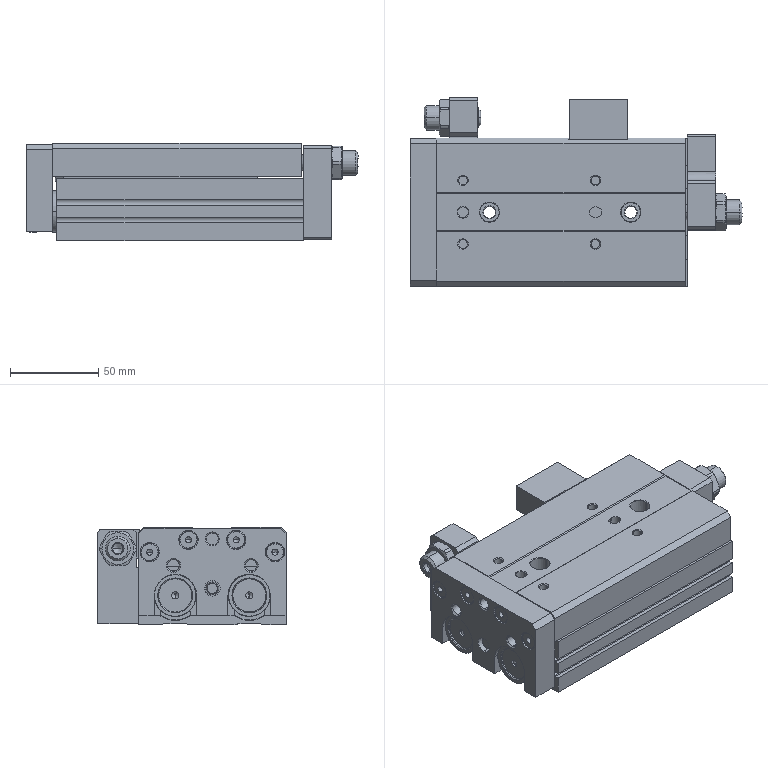Part | SolidWorks | 2 solids | 698 faces | box 188 x 107.01 x 55 mm | volume 634944 mm3 | plane 268 | cylinder 250 | cone 146 | spline 34 | commonest cylinder face diameters 6.647 x18 4.917 x16 10.5 x16 11 x16 6 x14 4 x12